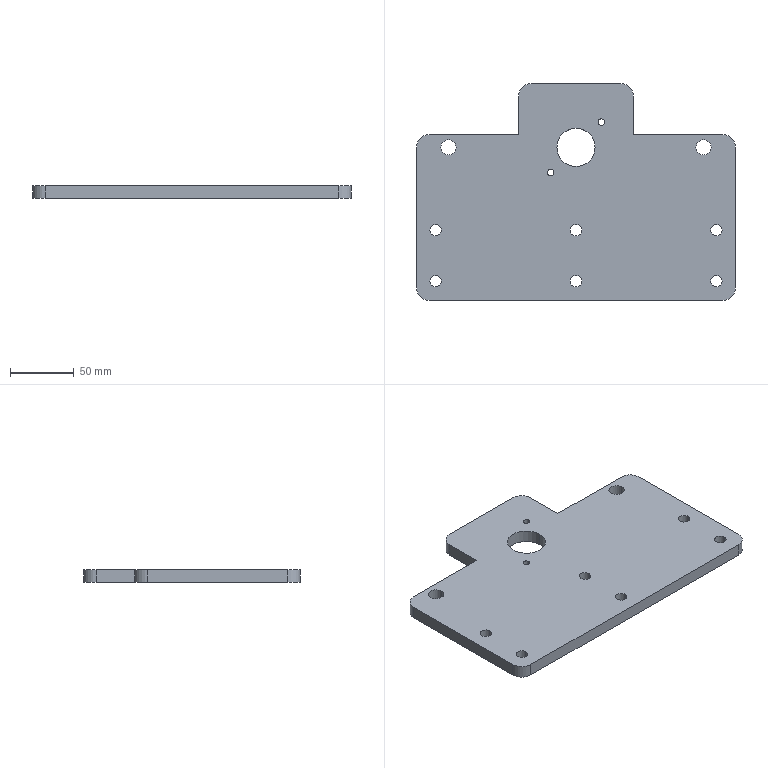Part | SolidWorks | features HoleWzd 3, ICE 2, Extrusion 1, Fillet 1, LPattern 1, MirrorPattern 1 | 1 solid | 38 faces | box 250 x 170 x 10 mm | volume 346172 mm3 | cylinder 28 | plane 10 | commonest cylinder face diameters 9 x12 20 x6 5 x4 12 x4 30 x2
STEP:
#1=CARTESIAN_POINT('',(-22.3,15.2,-5.));
#2=VERTEX_POINT('',#1);
#3=CARTESIAN_POINT('',(-17.3,15.2,-5.));
#4=VERTEX_POINT('',#3);
#5=CARTESIAN_POINT('',(-19.8,15.2,-5.));
#6=DIRECTION('',(0.,0.,1.));
#7=DIRECTION('',(1.,0.,0.));
#8=AXIS2_PLACEMENT_3D('',#5,#6,#7);
#9=CIRCLE('',#8,2.5);
#10=EDGE_CURVE('',#2,#4,#9,.T.);
#11=ORIENTED_EDGE('',*,*,#10,.F.);
#12=CARTESIAN_POINT('',(-22.3,15.2,5.));
#13=VERTEX_POINT('',#12);
#14=CARTESIAN_POINT('',(-22.3,15.2,5.));
#15=DIRECTION('',(0.,0.,1.));
#16=VECTOR('',#15,1000.);
#17=LINE('',#14,#16);
#18=EDGE_CURVE('',#2,#13,#17,.T.);
#19=ORIENTED_EDGE('',*,*,#18,.T.);
#20=CARTESIAN_POINT('',(-17.3,15.2,5.));
#21=VERTEX_POINT('',#20);
#22=CARTESIAN_POINT('',(-19.8,15.2,5.));
#23=DIRECTION('',(0.,0.,1.));
#24=DIRECTION('',(1.,0.,0.));
#25=AXIS2_PLACEMENT_3D('',#22,#23,#24);
#26=CIRCLE('',#25,2.5);
#27=EDGE_CURVE('',#13,#21,#26,.T.);
#28=ORIENTED_EDGE('',*,*,#27,.T.);
#29=CARTESIAN_POINT('',(-17.3,15.2,5.));
#30=DIRECTION('',(0.,0.,1.));
#31=VECTOR('',#30,1000.);
#32=LINE('',#29,#31);
#33=EDGE_CURVE('',#4,#21,#32,.T.);
#34=ORIENTED_EDGE('',*,*,#33,.F.);
#35=EDGE_LOOP('',(#11,#19,#28,#34));
#36=FACE_OUTER_BOUND('',#35,.T.);
#37=CARTESIAN_POINT('',(-19.8,15.2,5.));
#38=DIRECTION('',(0.,0.,1.));
#39=DIRECTION('',(1.,0.,0.));
#40=AXIS2_PLACEMENT_3D('',#37,#38,#39);
#41=CYLINDRICAL_SURFACE('',#40,2.5);
#42=ADVANCED_FACE('',(#36),#41,.F.);
#43=CARTESIAN_POINT('',(17.3,54.8,-5.));
#44=VERTEX_POINT('',#43);
#45=CARTESIAN_POINT('',(22.3,54.8,-5.));
#46=VERTEX_POINT('',#45);
#47=CARTESIAN_POINT('',(19.8,54.8,-5.));
#48=DIRECTION('',(0.,0.,1.));
#49=DIRECTION('',(1.,0.,0.));
#50=AXIS2_PLACEMENT_3D('',#47,#48,#49);
#51=CIRCLE('',#50,2.5);
#52=EDGE_CURVE('',#44,#46,#51,.T.);
#53=ORIENTED_EDGE('',*,*,#52,.F.);
#54=CARTESIAN_POINT('',(17.3,54.8,5.));
#55=VERTEX_POINT('',#54);
#56=CARTESIAN_POINT('',(17.3,54.8,5.));
#57=DIRECTION('',(0.,0.,1.));
#58=VECTOR('',#57,1000.);
#59=LINE('',#56,#58);
#60=EDGE_CURVE('',#44,#55,#59,.T.);
#61=ORIENTED_EDGE('',*,*,#60,.T.);
#62=CARTESIAN_POINT('',(22.3,54.8,5.));
#63=VERTEX_POINT('',#62);
#64=CARTESIAN_POINT('',(19.8,54.8,5.));
#65=DIRECTION('',(0.,0.,1.));
#66=DIRECTION('',(1.,0.,0.));
#67=AXIS2_PLACEMENT_3D('',#64,#65,#66);
#68=CIRCLE('',#67,2.5);
#69=EDGE_CURVE('',#55,#63,#68,.T.);
#70=ORIENTED_EDGE('',*,*,#69,.T.);
#71=CARTESIAN_POINT('',(22.3,54.8,5.));
#72=DIRECTION('',(0.,0.,1.));
#73=VECTOR('',#72,1000.);
#74=LINE('',#71,#73);
#75=EDGE_CURVE('',#46,#63,#74,.T.);
#76=ORIENTED_EDGE('',*,*,#75,.F.);
#77=EDGE_LOOP('',(#53,#61,#70,#76));
#78=FACE_OUTER_BOUND('',#77,.T.);
#79=CARTESIAN_POINT('',(19.8,54.8,5.));
#80=DIRECTION('',(0.,0.,1.));
#81=DIRECTION('',(1.,0.,0.));
#82=AXIS2_PLACEMENT_3D('',#79,#80,#81);
#83=CYLINDRICAL_SURFACE('',#82,2.5);
#84=ADVANCED_FACE('',(#78),#83,.F.);
#85=CARTESIAN_POINT('',(-15.,35.,-5.));
#86=VERTEX_POINT('',#85);
#87=CARTESIAN_POINT('',(15.,35.,-5.));
#88=VERTEX_POINT('',#87);
#89=CARTESIAN_POINT('',(0.,35.,-5.));
#90=DIRECTION('',(0.,0.,1.));
#91=DIRECTION('',(1.,0.,0.));
#92=AXIS2_PLACEMENT_3D('',#89,#90,#91);
#93=CIRCLE('',#92,15.);
#94=EDGE_CURVE('',#86,#88,#93,.T.);
#95=ORIENTED_EDGE('',*,*,#94,.F.);
#96=CARTESIAN_POINT('',(-15.,35.,5.));
#97=VERTEX_POINT('',#96);
#98=CARTESIAN_POINT('',(-15.,35.,-5.));
#99=DIRECTION('',(0.,0.,1.));
#100=VECTOR('',#99,1000.);
#101=LINE('',#98,#100);
#102=EDGE_CURVE('',#86,#97,#101,.T.);
#103=ORIENTED_EDGE('',*,*,#102,.T.);
#104=CARTESIAN_POINT('',(15.,35.,5.));
#105=VERTEX_POINT('',#104);
#106=CARTESIAN_POINT('',(0.,35.,5.));
#107=DIRECTION('',(0.,0.,1.));
#108=DIRECTION('',(1.,0.,0.));
#109=AXIS2_PLACEMENT_3D('',#106,#107,#108);
#110=CIRCLE('',#109,15.);
#111=EDGE_CURVE('',#97,#105,#110,.T.);
#112=ORIENTED_EDGE('',*,*,#111,.T.);
#113=CARTESIAN_POINT('',(15.,35.,-5.));
#114=DIRECTION('',(0.,0.,1.));
#115=VECTOR('',#114,1000.);
#116=LINE('',#113,#115);
#117=EDGE_CURVE('',#88,#105,#116,.T.);
#118=ORIENTED_EDGE('',*,*,#117,.F.);
#119=EDGE_LOOP('',(#95,#103,#112,#118));
#120=FACE_OUTER_BOUND('',#119,.T.);
#121=CARTESIAN_POINT('',(0.,35.,-5.));
#122=DIRECTION('',(0.,0.,1.));
#123=DIRECTION('',(1.,0.,0.));
#124=AXIS2_PLACEMENT_3D('',#121,#122,#123);
#125=CYLINDRICAL_SURFACE('',#124,15.);
#126=ADVANCED_FACE('',(#120),#125,.F.);
#127=CARTESIAN_POINT('',(-106.,35.,-5.));
#128=VERTEX_POINT('',#127);
#129=CARTESIAN_POINT('',(-94.,35.,-5.));
#130=VERTEX_POINT('',#129);
#131=CARTESIAN_POINT('',(-100.,35.,-5.));
#132=DIRECTION('',(0.,0.,1.));
#133=DIRECTION('',(1.,0.,0.));
#134=AXIS2_PLACEMENT_3D('',#131,#132,#133);
#135=CIRCLE('',#134,6.);
#136=EDGE_CURVE('',#128,#130,#135,.T.);
#137=ORIENTED_EDGE('',*,*,#136,.F.);
#138=CARTESIAN_POINT('',(-106.,35.,5.));
#139=VERTEX_POINT('',#138);
#140=CARTESIAN_POINT('',(-106.,35.,5.));
#141=DIRECTION('',(0.,0.,1.));
#142=VECTOR('',#141,1000.);
#143=LINE('',#140,#142);
#144=EDGE_CURVE('',#128,#139,#143,.T.);
#145=ORIENTED_EDGE('',*,*,#144,.T.);
#146=CARTESIAN_POINT('',(-94.,35.,5.));
#147=VERTEX_POINT('',#146);
#148=CARTESIAN_POINT('',(-100.,35.,5.));
#149=DIRECTION('',(0.,0.,1.));
#150=DIRECTION('',(1.,0.,0.));
#151=AXIS2_PLACEMENT_3D('',#148,#149,#150);
#152=CIRCLE('',#151,6.);
#153=EDGE_CURVE('',#139,#147,#152,.T.);
#154=ORIENTED_EDGE('',*,*,#153,.T.);
#155=CARTESIAN_POINT('',(-94.,35.,5.));
#156=DIRECTION('',(0.,0.,1.));
#157=VECTOR('',#156,1000.);
#158=LINE('',#155,#157);
#159=EDGE_CURVE('',#130,#147,#158,.T.);
#160=ORIENTED_EDGE('',*,*,#159,.F.);
#161=EDGE_LOOP('',(#137,#145,#154,#160));
#162=FACE_OUTER_BOUND('',#161,.T.);
#163=CARTESIAN_POINT('',(-100.,35.,5.));
#164=DIRECTION('',(0.,0.,1.));
#165=DIRECTION('',(1.,0.,0.));
#166=AXIS2_PLACEMENT_3D('',#163,#164,#165);
#167=CYLINDRICAL_SURFACE('',#166,6.);
#168=ADVANCED_FACE('',(#162),#167,.F.);
#169=CARTESIAN_POINT('',(94.,35.,-5.));
#170=VERTEX_POINT('',#169);
#171=CARTESIAN_POINT('',(106.,35.,-5.));
#172=VERTEX_POINT('',#171);
#173=CARTESIAN_POINT('',(100.,35.,-5.));
#174=DIRECTION('',(0.,0.,1.));
#175=DIRECTION('',(1.,0.,0.));
#176=AXIS2_PLACEMENT_3D('',#173,#174,#175);
#177=CIRCLE('',#176,6.);
#178=EDGE_CURVE('',#170,#172,#177,.T.);
#179=ORIENTED_EDGE('',*,*,#178,.F.);
#180=CARTESIAN_POINT('',(94.,35.,5.));
#181=VERTEX_POINT('',#180);
#182=CARTESIAN_POINT('',(94.,35.,5.));
#183=DIRECTION('',(0.,0.,1.));
#184=VECTOR('',#183,1000.);
#185=LINE('',#182,#184);
#186=EDGE_CURVE('',#170,#181,#185,.T.);
#187=ORIENTED_EDGE('',*,*,#186,.T.);
#188=CARTESIAN_POINT('',(106.,35.,5.));
#189=VERTEX_POINT('',#188);
#190=CARTESIAN_POINT('',(100.,35.,5.));
#191=DIRECTION('',(0.,0.,1.));
#192=DIRECTION('',(1.,0.,0.));
#193=AXIS2_PLACEMENT_3D('',#190,#191,#192);
#194=CIRCLE('',#193,6.);
#195=EDGE_CURVE('',#181,#189,#194,.T.);
#196=ORIENTED_EDGE('',*,*,#195,.T.);
#197=CARTESIAN_POINT('',(106.,35.,5.));
#198=DIRECTION('',(0.,0.,1.));
#199=VECTOR('',#198,1000.);
#200=LINE('',#197,#199);
#201=EDGE_CURVE('',#172,#189,#200,.T.);
#202=ORIENTED_EDGE('',*,*,#201,.F.);
#203=EDGE_LOOP('',(#179,#187,#196,#202));
#204=FACE_OUTER_BOUND('',#203,.T.);
#205=CARTESIAN_POINT('',(100.,35.,5.));
#206=DIRECTION('',(0.,0.,1.));
#207=DIRECTION('',(1.,0.,0.));
#208=AXIS2_PLACEMENT_3D('',#205,#206,#207);
#209=CYLINDRICAL_SURFACE('',#208,6.);
#210=ADVANCED_FACE('',(#204),#209,.F.);
#211=CARTESIAN_POINT('',(105.5,-70.,-5.));
#212=VERTEX_POINT('',#211);
#213=CARTESIAN_POINT('',(114.5,-70.,-5.));
#214=VERTEX_POINT('',#213);
#215=CARTESIAN_POINT('',(110.,-70.,-5.));
#216=DIRECTION('',(0.,0.,1.));
#217=DIRECTION('',(1.,0.,0.));
#218=AXIS2_PLACEMENT_3D('',#215,#216,#217);
#219=CIRCLE('',#218,4.5);
#220=EDGE_CURVE('',#212,#214,#219,.T.);
#221=ORIENTED_EDGE('',*,*,#220,.F.);
#222=CARTESIAN_POINT('',(105.5,-70.,5.));
#223=VERTEX_POINT('',#222);
#224=CARTESIAN_POINT('',(105.5,-70.,5.));
#225=DIRECTION('',(0.,0.,1.));
#226=VECTOR('',#225,1000.);
#227=LINE('',#224,#226);
#228=EDGE_CURVE('',#212,#223,#227,.T.);
#229=ORIENTED_EDGE('',*,*,#228,.T.);
#230=CARTESIAN_POINT('',(114.5,-70.,5.));
#231=VERTEX_POINT('',#230);
#232=CARTESIAN_POINT('',(110.,-70.,5.));
#233=DIRECTION('',(0.,0.,1.));
#234=DIRECTION('',(1.,0.,0.));
#235=AXIS2_PLACEMENT_3D('',#232,#233,#234);
#236=CIRCLE('',#235,4.5);
#237=EDGE_CURVE('',#223,#231,#236,.T.);
#238=ORIENTED_EDGE('',*,*,#237,.T.);
#239=CARTESIAN_POINT('',(114.5,-70.,5.));
#240=DIRECTION('',(0.,0.,1.));
#241=VECTOR('',#240,1000.);
#242=LINE('',#239,#241);
#243=EDGE_CURVE('',#214,#231,#242,.T.);
#244=ORIENTED_EDGE('',*,*,#243,.F.);
#245=EDGE_LOOP('',(#221,#229,#238,#244));
#246=FACE_OUTER_BOUND('',#245,.T.);
#247=CARTESIAN_POINT('',(110.,-70.,5.));
#248=DIRECTION('',(0.,0.,1.));
#249=DIRECTION('',(1.,0.,0.));
#250=AXIS2_PLACEMENT_3D('',#247,#248,#249);
#251=CYLINDRICAL_SURFACE('',#250,4.5);
#252=ADVANCED_FACE('',(#246),#251,.F.);
#253=CARTESIAN_POINT('',(-4.5,-70.,-5.));
#254=VERTEX_POINT('',#253);
#255=CARTESIAN_POINT('',(4.5,-70.,-5.));
#256=VERTEX_POINT('',#255);
#257=CARTESIAN_POINT('',(0.,-70.,-5.));
#258=DIRECTION('',(0.,0.,1.));
#259=DIRECTION('',(1.,0.,0.));
#260=AXIS2_PLACEMENT_3D('',#257,#258,#259);
#261=CIRCLE('',#260,4.5);
#262=EDGE_CURVE('',#254,#256,#261,.T.);
#263=ORIENTED_EDGE('',*,*,#262,.F.);
#264=CARTESIAN_POINT('',(-4.5,-70.,5.));
#265=VERTEX_POINT('',#264);
#266=CARTESIAN_POINT('',(-4.5,-70.,5.));
#267=DIRECTION('',(0.,0.,1.));
#268=VECTOR('',#267,1000.);
#269=LINE('',#266,#268);
#270=EDGE_CURVE('',#254,#265,#269,.T.);
#271=ORIENTED_EDGE('',*,*,#270,.T.);
#272=CARTESIAN_POINT('',(4.5,-70.,5.));
#273=VERTEX_POINT('',#272);
#274=CARTESIAN_POINT('',(0.,-70.,5.));
#275=DIRECTION('',(0.,0.,1.));
#276=DIRECTION('',(1.,0.,0.));
#277=AXIS2_PLACEMENT_3D('',#274,#275,#276);
#278=CIRCLE('',#277,4.5);
#279=EDGE_CURVE('',#265,#273,#278,.T.);
#280=ORIENTED_EDGE('',*,*,#279,.T.);
#281=CARTESIAN_POINT('',(4.5,-70.,5.));
#282=DIRECTION('',(0.,0.,1.));
#283=VECTOR('',#282,1000.);
#284=LINE('',#281,#283);
#285=EDGE_CURVE('',#256,#273,#284,.T.);
#286=ORIENTED_EDGE('',*,*,#285,.F.);
#287=EDGE_LOOP('',(#263,#271,#280,#286));
#288=FACE_OUTER_BOUND('',#287,.T.);
#289=CARTESIAN_POINT('',(0.,-70.,5.));
#290=DIRECTION('',(0.,0.,1.));
#291=DIRECTION('',(1.,0.,0.));
#292=AXIS2_PLACEMENT_3D('',#289,#290,#291);
#293=CYLINDRICAL_SURFACE('',#292,4.5);
#294=ADVANCED_FACE('',(#288),#293,.F.);
#295=CARTESIAN_POINT('',(105.5,-30.,-5.));
#296=VERTEX_POINT('',#295);
#297=CARTESIAN_POINT('',(114.5,-30.,-5.));
#298=VERTEX_POINT('',#297);
#299=CARTESIAN_POINT('',(110.,-30.,-5.));
#300=DIRECTION('',(0.,0.,1.));
#301=DIRECTION('',(1.,0.,0.));
#302=AXIS2_PLACEMENT_3D('',#299,#300,#301);
#303=CIRCLE('',#302,4.5);
#304=EDGE_CURVE('',#296,#298,#303,.T.);
#305=ORIENTED_EDGE('',*,*,#304,.F.);
#306=CARTESIAN_POINT('',(105.5,-30.,5.));
#307=VERTEX_POINT('',#306);
#308=CARTESIAN_POINT('',(105.5,-30.,5.));
#309=DIRECTION('',(0.,0.,1.));
#310=VECTOR('',#309,1000.);
#311=LINE('',#308,#310);
#312=EDGE_CURVE('',#296,#307,#311,.T.);
#313=ORIENTED_EDGE('',*,*,#312,.T.);
#314=CARTESIAN_POINT('',(114.5,-30.,5.));
#315=VERTEX_POINT('',#314);
#316=CARTESIAN_POINT('',(110.,-30.,5.));
#317=DIRECTION('',(0.,0.,1.));
#318=DIRECTION('',(1.,0.,0.));
#319=AXIS2_PLACEMENT_3D('',#316,#317,#318);
#320=CIRCLE('',#319,4.5);
#321=EDGE_CURVE('',#307,#315,#320,.T.);
#322=ORIENTED_EDGE('',*,*,#321,.T.);
#323=CARTESIAN_POINT('',(114.5,-30.,5.));
#324=DIRECTION('',(0.,0.,1.));
#325=VECTOR('',#324,1000.);
#326=LINE('',#323,#325);
#327=EDGE_CURVE('',#298,#315,#326,.T.);
#328=ORIENTED_EDGE('',*,*,#327,.F.);
#329=EDGE_LOOP('',(#305,#313,#322,#328));
#330=FACE_OUTER_BOUND('',#329,.T.);
#331=CARTESIAN_POINT('',(110.,-30.,5.));
#332=DIRECTION('',(0.,0.,1.));
#333=DIRECTION('',(1.,0.,0.));
#334=AXIS2_PLACEMENT_3D('',#331,#332,#333);
#335=CYLINDRICAL_SURFACE('',#334,4.5);
#336=ADVANCED_FACE('',(#330),#335,.F.);
#337=CARTESIAN_POINT('',(-4.5,-30.,-5.));
#338=VERTEX_POINT('',#337);
#339=CARTESIAN_POINT('',(4.5,-30.,-5.));
#340=VERTEX_POINT('',#339);
#341=CARTESIAN_POINT('',(0.,-30.,-5.));
#342=DIRECTION('',(0.,0.,1.));
#343=DIRECTION('',(1.,0.,0.));
#344=AXIS2_PLACEMENT_3D('',#341,#342,#343);
#345=CIRCLE('',#344,4.5);
#346=EDGE_CURVE('',#338,#340,#345,.T.);
#347=ORIENTED_EDGE('',*,*,#346,.F.);
#348=CARTESIAN_POINT('',(-4.5,-30.,5.));
#349=VERTEX_POINT('',#348);
#350=CARTESIAN_POINT('',(-4.5,-30.,5.));
#351=DIRECTION('',(0.,0.,1.));
#352=VECTOR('',#351,1000.);
#353=LINE('',#350,#352);
#354=EDGE_CURVE('',#338,#349,#353,.T.);
#355=ORIENTED_EDGE('',*,*,#354,.T.);
#356=CARTESIAN_POINT('',(4.5,-30.,5.));
#357=VERTEX_POINT('',#356);
#358=CARTESIAN_POINT('',(0.,-30.,5.));
#359=DIRECTION('',(0.,0.,1.));
#360=DIRECTION('',(1.,0.,0.));
#361=AXIS2_PLACEMENT_3D('',#358,#359,#360);
#362=CIRCLE('',#361,4.5);
#363=EDGE_CURVE('',#349,#357,#362,.T.);
#364=ORIENTED_EDGE('',*,*,#363,.T.);
#365=CARTESIAN_POINT('',(4.5,-30.,5.));
#366=DIRECTION('',(0.,0.,1.));
#367=VECTOR('',#366,1000.);
#368=LINE('',#365,#367);
#369=EDGE_CURVE('',#340,#357,#368,.T.);
#370=ORIENTED_EDGE('',*,*,#369,.F.);
#371=EDGE_LOOP('',(#347,#355,#364,#370));
#372=FACE_OUTER_BOUND('',#371,.T.);
#373=CARTESIAN_POINT('',(0.,-30.,5.));
#374=DIRECTION('',(0.,0.,1.));
#375=DIRECTION('',(1.,0.,0.));
#376=AXIS2_PLACEMENT_3D('',#373,#374,#375);
#377=CYLINDRICAL_SURFACE('',#376,4.5);
#378=ADVANCED_FACE('',(#372),#377,.F.);
#379=CARTESIAN_POINT('',(-114.5,-30.,-5.));
#380=VERTEX_POINT('',#379);
#381=CARTESIAN_POINT('',(-105.5,-30.,-5.));
#382=VERTEX_POINT('',#381);
#383=CARTESIAN_POINT('',(-110.,-30.,-5.));
#384=DIRECTION('',(0.,0.,1.));
#385=DIRECTION('',(1.,0.,0.));
#386=AXIS2_PLACEMENT_3D('',#383,#384,#385);
#387=CIRCLE('',#386,4.5);
#388=EDGE_CURVE('',#380,#382,#387,.T.);
#389=ORIENTED_EDGE('',*,*,#388,.F.);
#390=CARTESIAN_POINT('',(-114.5,-30.,5.));
#391=VERTEX_POINT('',#390);
#392=CARTESIAN_POINT('',(-114.5,-30.,5.));
#393=DIRECTION('',(0.,0.,1.));
#394=VECTOR('',#393,1000.);
#395=LINE('',#392,#394);
#396=EDGE_CURVE('',#380,#391,#395,.T.);
#397=ORIENTED_EDGE('',*,*,#396,.T.);
#398=CARTESIAN_POINT('',(-105.5,-30.,5.));
#399=VERTEX_POINT('',#398);
#400=CARTESIAN_POINT('',(-110.,-30.,5.));
#401=DIRECTION('',(0.,0.,1.));
#402=DIRECTION('',(1.,0.,0.));
#403=AXIS2_PLACEMENT_3D('',#400,#401,#402);
#404=CIRCLE('',#403,4.5);
#405=EDGE_CURVE('',#391,#399,#404,.T.);
#406=ORIENTED_EDGE('',*,*,#405,.T.);
#407=CARTESIAN_POINT('',(-105.5,-30.,5.));
#408=DIRECTION('',(0.,0.,1.));
#409=VECTOR('',#408,1000.);
#410=LINE('',#407,#409);
#411=EDGE_CURVE('',#382,#399,#410,.T.);
#412=ORIENTED_EDGE('',*,*,#411,.F.);
#413=EDGE_LOOP('',(#389,#397,#406,#412));
#414=FACE_OUTER_BOUND('',#413,.T.);
#415=CARTESIAN_POINT('',(-110.,-30.,5.));
#416=DIRECTION('',(0.,0.,1.));
#417=DIRECTION('',(1.,0.,0.));
#418=AXIS2_PLACEMENT_3D('',#415,#416,#417);
#419=CYLINDRICAL_SURFACE('',#418,4.5);
#420=ADVANCED_FACE('',(#414),#419,.F.);
#421=CARTESIAN_POINT('',(-114.5,-70.,-5.));
#422=VERTEX_POINT('',#421);
#423=CARTESIAN_POINT('',(-105.5,-70.,-5.));
#424=VERTEX_POINT('',#423);
#425=CARTESIAN_POINT('',(-110.,-70.,-5.));
#426=DIRECTION('',(0.,0.,1.));
#427=DIRECTION('',(1.,0.,0.));
#428=AXIS2_PLACEMENT_3D('',#425,#426,#427);
#429=CIRCLE('',#428,4.5);
#430=EDGE_CURVE('',#422,#424,#429,.T.);
#431=ORIENTED_EDGE('',*,*,#430,.F.);
#432=CARTESIAN_POINT('',(-114.5,-70.,5.));
#433=VERTEX_POINT('',#432);
#434=CARTESIAN_POINT('',(-114.5,-70.,5.));
#435=DIRECTION('',(0.,0.,1.));
#436=VECTOR('',#435,1000.);
#437=LINE('',#434,#436);
#438=EDGE_CURVE('',#422,#433,#437,.T.);
#439=ORIENTED_EDGE('',*,*,#438,.T.);
#440=CARTESIAN_POINT('',(-105.5,-70.,5.));
#441=VERTEX_POINT('',#440);
#442=CARTESIAN_POINT('',(-110.,-70.,5.));
#443=DIRECTION('',(0.,0.,1.));
#444=DIRECTION('',(1.,0.,0.));
#445=AXIS2_PLACEMENT_3D('',#442,#443,#444);
#446=CIRCLE('',#445,4.5);
#447=EDGE_CURVE('',#433,#441,#446,.T.);
#448=ORIENTED_EDGE('',*,*,#447,.T.);
#449=CARTESIAN_POINT('',(-105.5,-70.,5.));
#450=DIRECTION('',(0.,0.,1.));
#451=VECTOR('',#450,1000.);
#452=LINE('',#449,#451);
#453=EDGE_CURVE('',#424,#441,#452,.T.);
#454=ORIENTED_EDGE('',*,*,#453,.F.);
#455=EDGE_LOOP('',(#431,#439,#448,#454));
#456=FACE_OUTER_BOUND('',#455,.T.);
#457=CARTESIAN_POINT('',(-110.,-70.,5.));
#458=DIRECTION('',(0.,0.,1.));
#459=DIRECTION('',(1.,0.,0.));
#460=AXIS2_PLACEMENT_3D('',#457,#458,#459);
#461=CYLINDRICAL_SURFACE('',#460,4.5);
#462=ADVANCED_FACE('',(#456),#461,.F.);
#463=CARTESIAN_POINT('',(35.,85.,5.));
#464=VERTEX_POINT('',#463);
#465=CARTESIAN_POINT('',(-35.,85.,5.));
#466=VERTEX_POINT('',#465);
#467=CARTESIAN_POINT('',(-125.,85.,5.));
#468=DIRECTION('',(-1.,0.,0.));
#469=VECTOR('',#468,1000.);
#470=LINE('',#467,#469);
#471=EDGE_CURVE('',#464,#466,#470,.T.);
#472=ORIENTED_EDGE('',*,*,#471,.F.);
#473=CARTESIAN_POINT('',(35.,85.,-5.));
#474=VERTEX_POINT('',#473);
#475=CARTESIAN_POINT('',(35.,85.,5.));
#476=DIRECTION('',(0.,0.,-1.));
#477=VECTOR('',#476,1000.);
#478=LINE('',#475,#477);
#479=EDGE_CURVE('',#464,#474,#478,.T.);
#480=ORIENTED_EDGE('',*,*,#479,.T.);
#481=CARTESIAN_POINT('',(-35.,85.,-5.));
#482=VERTEX_POINT('',#481);
#483=CARTESIAN_POINT('',(-125.,85.,-5.));
#484=DIRECTION('',(-1.,0.,0.));
#485=VECTOR('',#484,1000.);
#486=LINE('',#483,#485);
#487=EDGE_CURVE('',#474,#482,#486,.T.);
#488=ORIENTED_EDGE('',*,*,#487,.T.);
#489=CARTESIAN_POINT('',(-35.,85.,5.));
#490=DIRECTION('',(0.,0.,1.));
#491=VECTOR('',#490,1000.);
#492=LINE('',#489,#491);
#493=EDGE_CURVE('',#482,#466,#492,.T.);
#494=ORIENTED_EDGE('',*,*,#493,.T.);
#495=EDGE_LOOP('',(#472,#480,#488,#494));
#496=FACE_OUTER_BOUND('',#495,.T.);
#497=CARTESIAN_POINT('',(-125.,85.,5.));
#498=DIRECTION('',(0.,-1.,0.));
#499=DIRECTION('',(0.,0.,-1.));
#500=AXIS2_PLACEMENT_3D('',#497,#498,#499);
#501=PLANE('',#500);
#502=ADVANCED_FACE('',(#496),#501,.F.);
#503=CARTESIAN_POINT('',(-125.,35.,-5.));
#504=VERTEX_POINT('',#503);
#505=CARTESIAN_POINT('',(-125.,-75.,-5.));
#506=VERTEX_POINT('',#505);
#507=CARTESIAN_POINT('',(-125.,85.,-5.));
#508=DIRECTION('',(0.,-1.,0.));
#509=VECTOR('',#508,1000.);
#510=LINE('',#507,#509);
#511=EDGE_CURVE('',#504,#506,#510,.T.);
#512=ORIENTED_EDGE('',*,*,#511,.T.);
#513=CARTESIAN_POINT('',(-125.,-75.,5.));
#514=VERTEX_POINT('',#513);
#515=CARTESIAN_POINT('',(-125.,-75.,5.));
#516=DIRECTION('',(0.,0.,1.));
#517=VECTOR('',#516,1000.);
#518=LINE('',#515,#517);
#519=EDGE_CURVE('',#506,#514,#518,.T.);
#520=ORIENTED_EDGE('',*,*,#519,.T.);
#521=CARTESIAN_POINT('',(-125.,35.,5.));
#522=VERTEX_POINT('',#521);
#523=CARTESIAN_POINT('',(-125.,85.,5.));
#524=DIRECTION('',(0.,-1.,0.));
#525=VECTOR('',#524,1000.);
#526=LINE('',#523,#525);
#527=EDGE_CURVE('',#522,#514,#526,.T.);
#528=ORIENTED_EDGE('',*,*,#527,.F.);
#529=CARTESIAN_POINT('',(-125.,35.,-5.));
#530=DIRECTION('',(0.,0.,-1.));
#531=VECTOR('',#530,1000.);
#532=LINE('',#529,#531);
#533=EDGE_CURVE('',#522,#504,#532,.T.);
#534=ORIENTED_EDGE('',*,*,#533,.T.);
#535=EDGE_LOOP('',(#512,#520,#528,#534));
#536=FACE_OUTER_BOUND('',#535,.T.);
#537=CARTESIAN_POINT('',(-125.,85.,5.));
#538=DIRECTION('',(1.,0.,0.));
#539=DIRECTION('',(0.,1.,0.));
#540=AXIS2_PLACEMENT_3D('',#537,#538,#539);
#541=PLANE('',#540);
#542=ADVANCED_FACE('',(#536),#541,.F.);
#543=CARTESIAN_POINT('',(-19.8,15.2,5.));
#544=DIRECTION('',(0.,0.,1.));
#545=DIRECTION('',(1.,0.,0.));
#546=AXIS2_PLACEMENT_3D('',#543,#544,#545);
#547=CIRCLE('',#546,2.5);
#548=EDGE_CURVE('',#21,#13,#547,.T.);
#549=ORIENTED_EDGE('',*,*,#548,.F.);
#550=ORIENTED_EDGE('',*,*,#27,.F.);
#551=EDGE_LOOP('',(#549,#550));
#552=FACE_BOUND('',#551,.T.);
#553=CARTESIAN_POINT('',(19.8,54.8,5.));
#554=DIRECTION('',(0.,0.,1.));
#555=DIRECTION('',(1.,0.,0.));
#556=AXIS2_PLACEMENT_3D('',#553,#554,#555);
#557=CIRCLE('',#556,2.5);
#558=EDGE_CURVE('',#63,#55,#557,.T.);
#559=ORIENTED_EDGE('',*,*,#558,.F.);
#560=ORIENTED_EDGE('',*,*,#69,.F.);
#561=EDGE_LOOP('',(#559,#560));
#562=FACE_BOUND('',#561,.T.);
#563=CARTESIAN_POINT('',(0.,35.,5.));
#564=DIRECTION('',(0.,0.,1.));
#565=DIRECTION('',(1.,0.,0.));
#566=AXIS2_PLACEMENT_3D('',#563,#564,#565);
#567=CIRCLE('',#566,15.);
#568=EDGE_CURVE('',#105,#97,#567,.T.);
#569=ORIENTED_EDGE('',*,*,#568,.F.);
#570=ORIENTED_EDGE('',*,*,#111,.F.);
#571=EDGE_LOOP('',(#569,#570));
#572=FACE_BOUND('',#571,.T.);
#573=CARTESIAN_POINT('',(-100.,35.,5.));
#574=DIRECTION('',(0.,0.,1.));
#575=DIRECTION('',(1.,0.,0.));
#576=AXIS2_PLACEMENT_3D('',#573,#574,#575);
#577=CIRCLE('',#576,6.);
#578=EDGE_CURVE('',#147,#139,#577,.T.);
#579=ORIENTED_EDGE('',*,*,#578,.F.);
#580=ORIENTED_EDGE('',*,*,#153,.F.);
#581=EDGE_LOOP('',(#579,#580));
#582=FACE_BOUND('',#581,.T.);
#583=CARTESIAN_POINT('',(100.,35.,5.));
#584=DIRECTION('',(0.,0.,1.));
#585=DIRECTION('',(1.,0.,0.));
#586=AXIS2_PLACEMENT_3D('',#583,#584,#585);
#587=CIRCLE('',#586,6.);
#588=EDGE_CURVE('',#189,#181,#587,.T.);
#589=ORIENTED_EDGE('',*,*,#588,.F.);
#590=ORIENTED_EDGE('',*,*,#195,.F.);
#591=EDGE_LOOP('',(#589,#590));
#592=FACE_BOUND('',#591,.T.);
#593=CARTESIAN_POINT('',(0.,-70.,5.));
#594=DIRECTION('',(0.,0.,1.));
#595=DIRECTION('',(1.,0.,0.));
#596=AXIS2_PLACEMENT_3D('',#593,#594,#595);
#597=CIRCLE('',#596,4.5);
#598=EDGE_CURVE('',#273,#265,#597,.T.);
#599=ORIENTED_EDGE('',*,*,#598,.F.);
#600=ORIENTED_EDGE('',*,*,#279,.F.);
#601=EDGE_LOOP('',(#599,#600));
#602=FACE_BOUND('',#601,.T.);
#603=CARTESIAN_POINT('',(0.,-30.,5.));
#604=DIRECTION('',(0.,0.,1.));
#605=DIRECTION('',(1.,0.,0.));
#606=AXIS2_PLACEMENT_3D('',#603,#604,#605);
#607=CIRCLE('',#606,4.5);
#608=EDGE_CURVE('',#357,#349,#607,.T.);
#609=ORIENTED_EDGE('',*,*,#608,.F.);
#610=ORIENTED_EDGE('',*,*,#363,.F.);
#611=EDGE_LOOP('',(#609,#610));
#612=FACE_BOUND('',#611,.T.);
#613=CARTESIAN_POINT('',(-110.,-30.,5.));
#614=DIRECTION('',(0.,0.,1.));
#615=DIRECTION('',(1.,0.,0.));
#616=AXIS2_PLACEMENT_3D('',#613,#614,#615);
#617=CIRCLE('',#616,4.5);
#618=EDGE_CURVE('',#399,#391,#617,.T.);
#619=ORIENTED_EDGE('',*,*,#618,.F.);
#620=ORIENTED_EDGE('',*,*,#405,.F.);
#621=EDGE_LOOP('',(#619,#620));
#622=FACE_BOUND('',#621,.T.);
#623=CARTESIAN_POINT('',(-110.,-70.,5.));
#624=DIRECTION('',(0.,0.,1.));
#625=DIRECTION('',(1.,0.,0.));
#626=AXIS2_PLACEMENT_3D('',#623,#624,#625);
#627=CIRCLE('',#626,4.5);
#628=EDGE_CURVE('',#441,#433,#627,.T.);
#629=ORIENTED_EDGE('',*,*,#628,.F.);
#630=ORIENTED_EDGE('',*,*,#447,.F.);
#631=EDGE_LOOP('',(#629,#630));
#632=FACE_BOUND('',#631,.T.);
#633=CARTESIAN_POINT('',(-115.,-85.,5.));
#634=VERTEX_POINT('',#633);
#635=CARTESIAN_POINT('',(115.,-85.,5.));
#636=VERTEX_POINT('',#635);
#637=CARTESIAN_POINT('',(-125.,-85.,5.));
#638=DIRECTION('',(1.,0.,0.));
#639=VECTOR('',#638,1000.);
#640=LINE('',#637,#639);
#641=EDGE_CURVE('',#634,#636,#640,.T.);
#642=ORIENTED_EDGE('',*,*,#641,.T.);
#643=CARTESIAN_POINT('',(125.,-75.,5.));
#644=VERTEX_POINT('',#643);
#645=CARTESIAN_POINT('',(115.,-75.,5.));
#646=DIRECTION('',(0.,0.,1.));
#647=DIRECTION('',(1.,0.,0.));
#648=AXIS2_PLACEMENT_3D('',#645,#646,#647);
#649=CIRCLE('',#648,10.);
#650=EDGE_CURVE('',#636,#644,#649,.T.);
#651=ORIENTED_EDGE('',*,*,#650,.T.);
#652=CARTESIAN_POINT('',(125.,35.,5.));
#653=VERTEX_POINT('',#652);
#654=CARTESIAN_POINT('',(125.,85.,5.));
#655=DIRECTION('',(0.,1.,0.));
#656=VECTOR('',#655,1000.);
#657=LINE('',#654,#656);
#658=EDGE_CURVE('',#644,#653,#657,.T.);
#659=ORIENTED_EDGE('',*,*,#658,.T.);
#660=CARTESIAN_POINT('',(115.,45.,5.));
#661=VERTEX_POINT('',#660);
#662=CARTESIAN_POINT('',(115.,35.,5.));
#663=DIRECTION('',(0.,0.,1.));
#664=DIRECTION('',(1.,0.,0.));
#665=AXIS2_PLACEMENT_3D('',#662,#663,#664);
#666=CIRCLE('',#665,10.);
#667=EDGE_CURVE('',#653,#661,#666,.T.);
#668=ORIENTED_EDGE('',*,*,#667,.T.);
#669=CARTESIAN_POINT('',(45.,45.,5.));
#670=VERTEX_POINT('',#669);
#671=CARTESIAN_POINT('',(45.,45.,5.));
#672=DIRECTION('',(1.,0.,0.));
#673=VECTOR('',#672,1000.);
#674=LINE('',#671,#673);
#675=EDGE_CURVE('',#670,#661,#674,.T.);
#676=ORIENTED_EDGE('',*,*,#675,.F.);
#677=CARTESIAN_POINT('',(45.,75.,5.));
#678=VERTEX_POINT('',#677);
#679=CARTESIAN_POINT('',(45.,85.,5.));
#680=DIRECTION('',(0.,-1.,0.));
#681=VECTOR('',#680,1000.);
#682=LINE('',#679,#681);
#683=EDGE_CURVE('',#678,#670,#682,.T.);
#684=ORIENTED_EDGE('',*,*,#683,.F.);
#685=CARTESIAN_POINT('',(35.,75.,5.));
#686=DIRECTION('',(0.,0.,1.));
#687=DIRECTION('',(1.,0.,0.));
#688=AXIS2_PLACEMENT_3D('',#685,#686,#687);
#689=CIRCLE('',#688,10.);
#690=EDGE_CURVE('',#678,#464,#689,.T.);
#691=ORIENTED_EDGE('',*,*,#690,.T.);
#692=ORIENTED_EDGE('',*,*,#471,.T.);
#693=CARTESIAN_POINT('',(-45.,75.,5.));
#694=VERTEX_POINT('',#693);
#695=CARTESIAN_POINT('',(-35.,75.,5.));
#696=DIRECTION('',(0.,0.,1.));
#697=DIRECTION('',(1.,0.,0.));
#698=AXIS2_PLACEMENT_3D('',#695,#696,#697);
#699=CIRCLE('',#698,10.);
#700=EDGE_CURVE('',#466,#694,#699,.T.);
#701=ORIENTED_EDGE('',*,*,#700,.T.);
#702=CARTESIAN_POINT('',(-45.,45.,5.));
#703=VERTEX_POINT('',#702);
#704=CARTESIAN_POINT('',(-45.,85.,5.));
#705=DIRECTION('',(0.,-1.,0.));
#706=VECTOR('',#705,1000.);
#707=LINE('',#704,#706);
#708=EDGE_CURVE('',#694,#703,#707,.T.);
#709=ORIENTED_EDGE('',*,*,#708,.T.);
#710=CARTESIAN_POINT('',(-115.,45.,5.));
#711=VERTEX_POINT('',#710);
#712=CARTESIAN_POINT('',(-45.,45.,5.));
#713=DIRECTION('',(-1.,0.,0.));
#714=VECTOR('',#713,1000.);
#715=LINE('',#712,#714);
#716=EDGE_CURVE('',#703,#711,#715,.T.);
#717=ORIENTED_EDGE('',*,*,#716,.T.);
#718=CARTESIAN_POINT('',(-115.,35.,5.));
#719=DIRECTION('',(0.,0.,1.));
#720=DIRECTION('',(1.,0.,0.));
#721=AXIS2_PLACEMENT_3D('',#718,#719,#720);
#722=CIRCLE('',#721,10.);
#723=EDGE_CURVE('',#711,#522,#722,.T.);
#724=ORIENTED_EDGE('',*,*,#723,.T.);
#725=ORIENTED_EDGE('',*,*,#527,.T.);
#726=CARTESIAN_POINT('',(-115.,-75.,5.));
#727=DIRECTION('',(0.,0.,1.));
#728=DIRECTION('',(1.,0.,0.));
#729=AXIS2_PLACEMENT_3D('',#726,#727,#728);
#730=CIRCLE('',#729,10.);
#731=EDGE_CURVE('',#514,#634,#730,.T.);
#732=ORIENTED_EDGE('',*,*,#731,.T.);
#733=EDGE_LOOP('',(#642,#651,#659,#668,#676,#684,#691,#692,#701,#709,#717,#724,#725,#732));
#734=FACE_OUTER_BOUND('',#733,.T.);
#735=CARTESIAN_POINT('',(110.,-30.,5.));
#736=DIRECTION('',(0.,0.,1.));
#737=DIRECTION('',(1.,0.,0.));
#738=AXIS2_PLACEMENT_3D('',#735,#736,#737);
#739=CIRCLE('',#738,4.5);
#740=EDGE_CURVE('',#315,#307,#739,.T.);
#741=ORIENTED_EDGE('',*,*,#740,.F.);
#742=ORIENTED_EDGE('',*,*,#321,.F.);
#743=EDGE_LOOP('',(#741,#742));
#744=FACE_BOUND('',#743,.T.);
#745=CARTESIAN_POINT('',(110.,-70.,5.));
#746=DIRECTION('',(0.,0.,1.));
#747=DIRECTION('',(1.,0.,0.));
#748=AXIS2_PLACEMENT_3D('',#745,#746,#747);
#749=CIRCLE('',#748,4.5);
#750=EDGE_CURVE('',#231,#223,#749,.T.);
#751=ORIENTED_EDGE('',*,*,#750,.F.);
#752=ORIENTED_EDGE('',*,*,#237,.F.);
#753=EDGE_LOOP('',(#751,#752));
#754=FACE_BOUND('',#753,.T.);
#755=CARTESIAN_POINT('',(0.,0.,5.));
#756=DIRECTION('',(0.,0.,1.));
#757=DIRECTION('',(1.,0.,0.));
#758=AXIS2_PLACEMENT_3D('',#755,#756,#757);
#759=PLANE('',#758);
#760=ADVANCED_FACE('',(#552,#562,#572,#582,#592,#602,#612,#622,#632,#734,#744,#754),#759,.T.);
#761=CARTESIAN_POINT('',(-19.8,15.2,-5.));
#762=DIRECTION('',(0.,0.,1.));
#763=DIRECTION('',(1.,0.,0.));
#764=AXIS2_PLACEMENT_3D('',#761,#762,#763);
#765=CIRCLE('',#764,2.5);
#766=EDGE_CURVE('',#4,#2,#765,.T.);
#767=ORIENTED_EDGE('',*,*,#766,.T.);
#768=ORIENTED_EDGE('',*,*,#10,.T.);
#769=EDGE_LOOP('',(#767,#768));
#770=FACE_BOUND('',#769,.T.);
#771=CARTESIAN_POINT('',(19.8,54.8,-5.));
#772=DIRECTION('',(0.,0.,1.));
#773=DIRECTION('',(1.,0.,0.));
#774=AXIS2_PLACEMENT_3D('',#771,#772,#773);
#775=CIRCLE('',#774,2.5);
#776=EDGE_CURVE('',#46,#44,#775,.T.);
#777=ORIENTED_EDGE('',*,*,#776,.T.);
#778=ORIENTED_EDGE('',*,*,#52,.T.);
#779=EDGE_LOOP('',(#777,#778));
#780=FACE_BOUND('',#779,.T.);
#781=CARTESIAN_POINT('',(0.,35.,-5.));
#782=DIRECTION('',(0.,0.,1.));
#783=DIRECTION('',(1.,0.,0.));
#784=AXIS2_PLACEMENT_3D('',#781,#782,#783);
#785=CIRCLE('',#784,15.);
#786=EDGE_CURVE('',#88,#86,#785,.T.);
#787=ORIENTED_EDGE('',*,*,#786,.T.);
#788=ORIENTED_EDGE('',*,*,#94,.T.);
#789=EDGE_LOOP('',(#787,#788));
#790=FACE_BOUND('',#789,.T.);
#791=CARTESIAN_POINT('',(-100.,35.,-5.));
#792=DIRECTION('',(0.,0.,1.));
#793=DIRECTION('',(1.,0.,0.));
#794=AXIS2_PLACEMENT_3D('',#791,#792,#793);
#795=CIRCLE('',#794,6.);
#796=EDGE_CURVE('',#130,#128,#795,.T.);
#797=ORIENTED_EDGE('',*,*,#796,.T.);
#798=ORIENTED_EDGE('',*,*,#136,.T.);
#799=EDGE_LOOP('',(#797,#798));
#800=FACE_BOUND('',#799,.T.);
#801=CARTESIAN_POINT('',(100.,35.,-5.));
#802=DIRECTION('',(0.,0.,1.));
#803=DIRECTION('',(1.,0.,0.));
#804=AXIS2_PLACEMENT_3D('',#801,#802,#803);
#805=CIRCLE('',#804,6.);
#806=EDGE_CURVE('',#172,#170,#805,.T.);
#807=ORIENTED_EDGE('',*,*,#806,.T.);
#808=ORIENTED_EDGE('',*,*,#178,.T.);
#809=EDGE_LOOP('',(#807,#808));
#810=FACE_BOUND('',#809,.T.);
#811=CARTESIAN_POINT('',(0.,-70.,-5.));
#812=DIRECTION('',(0.,0.,1.));
#813=DIRECTION('',(1.,0.,0.));
#814=AXIS2_PLACEMENT_3D('',#811,#812,#813);
#815=CIRCLE('',#814,4.5);
#816=EDGE_CURVE('',#256,#254,#815,.T.);
#817=ORIENTED_EDGE('',*,*,#816,.T.);
#818=ORIENTED_EDGE('',*,*,#262,.T.);
#819=EDGE_LOOP('',(#817,#818));
#820=FACE_BOUND('',#819,.T.);
#821=CARTESIAN_POINT('',(0.,-30.,-5.));
#822=DIRECTION('',(0.,0.,1.));
#823=DIRECTION('',(1.,0.,0.));
#824=AXIS2_PLACEMENT_3D('',#821,#822,#823);
#825=CIRCLE('',#824,4.5);
#826=EDGE_CURVE('',#340,#338,#825,.T.);
#827=ORIENTED_EDGE('',*,*,#826,.T.);
#828=ORIENTED_EDGE('',*,*,#346,.T.);
#829=EDGE_LOOP('',(#827,#828));
#830=FACE_BOUND('',#829,.T.);
#831=CARTESIAN_POINT('',(-110.,-30.,-5.));
#832=DIRECTION('',(0.,0.,1.));
#833=DIRECTION('',(1.,0.,0.));
#834=AXIS2_PLACEMENT_3D('',#831,#832,#833);
#835=CIRCLE('',#834,4.5);
#836=EDGE_CURVE('',#382,#380,#835,.T.);
#837=ORIENTED_EDGE('',*,*,#836,.T.);
#838=ORIENTED_EDGE('',*,*,#388,.T.);
#839=EDGE_LOOP('',(#837,#838));
#840=FACE_BOUND('',#839,.T.);
#841=CARTESIAN_POINT('',(-110.,-70.,-5.));
#842=DIRECTION('',(0.,0.,1.));
#843=DIRECTION('',(1.,0.,0.));
#844=AXIS2_PLACEMENT_3D('',#841,#842,#843);
#845=CIRCLE('',#844,4.5);
#846=EDGE_CURVE('',#424,#422,#845,.T.);
#847=ORIENTED_EDGE('',*,*,#846,.T.);
#848=ORIENTED_EDGE('',*,*,#430,.T.);
#849=EDGE_LOOP('',(#847,#848));
#850=FACE_BOUND('',#849,.T.);
#851=CARTESIAN_POINT('',(125.,-75.,-5.));
#852=VERTEX_POINT('',#851);
#853=CARTESIAN_POINT('',(125.,35.,-5.));
#854=VERTEX_POINT('',#853);
#855=CARTESIAN_POINT('',(125.,85.,-5.));
#856=DIRECTION('',(0.,1.,0.));
#857=VECTOR('',#856,1000.);
#858=LINE('',#855,#857);
#859=EDGE_CURVE('',#852,#854,#858,.T.);
#860=ORIENTED_EDGE('',*,*,#859,.F.);
#861=CARTESIAN_POINT('',(115.,-85.,-5.));
#862=VERTEX_POINT('',#861);
#863=CARTESIAN_POINT('',(115.,-75.,-5.));
#864=DIRECTION('',(0.,0.,-1.));
#865=DIRECTION('',(1.,0.,0.));
#866=AXIS2_PLACEMENT_3D('',#863,#864,#865);
#867=CIRCLE('',#866,10.);
#868=EDGE_CURVE('',#852,#862,#867,.T.);
#869=ORIENTED_EDGE('',*,*,#868,.T.);
#870=CARTESIAN_POINT('',(-115.,-85.,-5.));
#871=VERTEX_POINT('',#870);
#872=CARTESIAN_POINT('',(-125.,-85.,-5.));
#873=DIRECTION('',(1.,0.,0.));
#874=VECTOR('',#873,1000.);
#875=LINE('',#872,#874);
#876=EDGE_CURVE('',#871,#862,#875,.T.);
#877=ORIENTED_EDGE('',*,*,#876,.F.);
#878=CARTESIAN_POINT('',(-115.,-75.,-5.));
#879=DIRECTION('',(0.,0.,-1.));
#880=DIRECTION('',(1.,0.,0.));
#881=AXIS2_PLACEMENT_3D('',#878,#879,#880);
#882=CIRCLE('',#881,10.);
#883=EDGE_CURVE('',#871,#506,#882,.T.);
#884=ORIENTED_EDGE('',*,*,#883,.T.);
#885=ORIENTED_EDGE('',*,*,#511,.F.);
#886=CARTESIAN_POINT('',(-115.,45.,-5.));
#887=VERTEX_POINT('',#886);
#888=CARTESIAN_POINT('',(-115.,35.,-5.));
#889=DIRECTION('',(0.,0.,-1.));
#890=DIRECTION('',(1.,0.,0.));
#891=AXIS2_PLACEMENT_3D('',#888,#889,#890);
#892=CIRCLE('',#891,10.);
#893=EDGE_CURVE('',#504,#887,#892,.T.);
#894=ORIENTED_EDGE('',*,*,#893,.T.);
#895=CARTESIAN_POINT('',(-45.,45.,-5.));
#896=VERTEX_POINT('',#895);
#897=CARTESIAN_POINT('',(-45.,45.,-5.));
#898=DIRECTION('',(-1.,0.,0.));
#899=VECTOR('',#898,1000.);
#900=LINE('',#897,#899);
#901=EDGE_CURVE('',#896,#887,#900,.T.);
#902=ORIENTED_EDGE('',*,*,#901,.F.);
#903=CARTESIAN_POINT('',(-45.,75.,-5.));
#904=VERTEX_POINT('',#903);
#905=CARTESIAN_POINT('',(-45.,85.,-5.));
#906=DIRECTION('',(0.,-1.,0.));
#907=VECTOR('',#906,1000.);
#908=LINE('',#905,#907);
#909=EDGE_CURVE('',#904,#896,#908,.T.);
#910=ORIENTED_EDGE('',*,*,#909,.F.);
#911=CARTESIAN_POINT('',(-35.,75.,-5.));
#912=DIRECTION('',(0.,0.,-1.));
#913=DIRECTION('',(1.,0.,0.));
#914=AXIS2_PLACEMENT_3D('',#911,#912,#913);
#915=CIRCLE('',#914,10.);
#916=EDGE_CURVE('',#904,#482,#915,.T.);
#917=ORIENTED_EDGE('',*,*,#916,.T.);
#918=ORIENTED_EDGE('',*,*,#487,.F.);
#919=CARTESIAN_POINT('',(45.,75.,-5.));
#920=VERTEX_POINT('',#919);
#921=CARTESIAN_POINT('',(35.,75.,-5.));
#922=DIRECTION('',(0.,0.,-1.));
#923=DIRECTION('',(1.,0.,0.));
#924=AXIS2_PLACEMENT_3D('',#921,#922,#923);
#925=CIRCLE('',#924,10.);
#926=EDGE_CURVE('',#474,#920,#925,.T.);
#927=ORIENTED_EDGE('',*,*,#926,.T.);
#928=CARTESIAN_POINT('',(45.,45.,-5.));
#929=VERTEX_POINT('',#928);
#930=CARTESIAN_POINT('',(45.,85.,-5.));
#931=DIRECTION('',(0.,-1.,0.));
#932=VECTOR('',#931,1000.);
#933=LINE('',#930,#932);
#934=EDGE_CURVE('',#920,#929,#933,.T.);
#935=ORIENTED_EDGE('',*,*,#934,.T.);
#936=CARTESIAN_POINT('',(115.,45.,-5.));
#937=VERTEX_POINT('',#936);
#938=CARTESIAN_POINT('',(45.,45.,-5.));
#939=DIRECTION('',(1.,0.,0.));
#940=VECTOR('',#939,1000.);
#941=LINE('',#938,#940);
#942=EDGE_CURVE('',#929,#937,#941,.T.);
#943=ORIENTED_EDGE('',*,*,#942,.T.);
#944=CARTESIAN_POINT('',(115.,35.,-5.));
#945=DIRECTION('',(0.,0.,-1.));
#946=DIRECTION('',(1.,0.,0.));
#947=AXIS2_PLACEMENT_3D('',#944,#945,#946);
#948=CIRCLE('',#947,10.);
#949=EDGE_CURVE('',#937,#854,#948,.T.);
#950=ORIENTED_EDGE('',*,*,#949,.T.);
#951=EDGE_LOOP('',(#860,#869,#877,#884,#885,#894,#902,#910,#917,#918,#927,#935,#943,#950));
#952=FACE_OUTER_BOUND('',#951,.T.);
#953=CARTESIAN_POINT('',(110.,-30.,-5.));
#954=DIRECTION('',(0.,0.,1.));
#955=DIRECTION('',(1.,0.,0.));
#956=AXIS2_PLACEMENT_3D('',#953,#954,#955);
#957=CIRCLE('',#956,4.5);
#958=EDGE_CURVE('',#298,#296,#957,.T.);
#959=ORIENTED_EDGE('',*,*,#958,.T.);
#960=ORIENTED_EDGE('',*,*,#304,.T.);
#961=EDGE_LOOP('',(#959,#960));
#962=FACE_BOUND('',#961,.T.);
#963=CARTESIAN_POINT('',(110.,-70.,-5.));
#964=DIRECTION('',(0.,0.,1.));
#965=DIRECTION('',(1.,0.,0.));
#966=AXIS2_PLACEMENT_3D('',#963,#964,#965);
#967=CIRCLE('',#966,4.5);
#968=EDGE_CURVE('',#214,#212,#967,.T.);
#969=ORIENTED_EDGE('',*,*,#968,.T.);
#970=ORIENTED_EDGE('',*,*,#220,.T.);
#971=EDGE_LOOP('',(#969,#970));
#972=FACE_BOUND('',#971,.T.);
#973=CARTESIAN_POINT('',(0.,0.,-5.));
#974=DIRECTION('',(0.,0.,1.));
#975=DIRECTION('',(1.,0.,0.));
#976=AXIS2_PLACEMENT_3D('',#973,#974,#975);
#977=PLANE('',#976);
#978=ADVANCED_FACE('',(#770,#780,#790,#800,#810,#820,#830,#840,#850,#952,#962,#972),#977,.F.);
#979=ORIENTED_EDGE('',*,*,#658,.F.);
#980=CARTESIAN_POINT('',(125.,-75.,5.));
#981=DIRECTION('',(0.,0.,-1.));
#982=VECTOR('',#981,1000.);
#983=LINE('',#980,#982);
#984=EDGE_CURVE('',#644,#852,#983,.T.);
#985=ORIENTED_EDGE('',*,*,#984,.T.);
#986=ORIENTED_EDGE('',*,*,#859,.T.);
#987=CARTESIAN_POINT('',(125.,35.,5.));
#988=DIRECTION('',(0.,0.,1.));
#989=VECTOR('',#988,1000.);
#990=LINE('',#987,#989);
#991=EDGE_CURVE('',#854,#653,#990,.T.);
#992=ORIENTED_EDGE('',*,*,#991,.T.);
#993=EDGE_LOOP('',(#979,#985,#986,#992));
#994=FACE_OUTER_BOUND('',#993,.T.);
#995=CARTESIAN_POINT('',(125.,85.,5.));
#996=DIRECTION('',(-1.,0.,0.));
#997=DIRECTION('',(0.,0.,1.));
#998=AXIS2_PLACEMENT_3D('',#995,#996,#997);
#999=PLANE('',#998);
#1000=ADVANCED_FACE('',(#994),#999,.F.);
#1001=ORIENTED_EDGE('',*,*,#876,.T.);
#1002=CARTESIAN_POINT('',(115.,-85.,5.));
#1003=DIRECTION('',(0.,0.,1.));
#1004=VECTOR('',#1003,1000.);
#1005=LINE('',#1002,#1004);
#1006=EDGE_CURVE('',#862,#636,#1005,.T.);
#1007=ORIENTED_EDGE('',*,*,#1006,.T.);
#1008=ORIENTED_EDGE('',*,*,#641,.F.);
#1009=CARTESIAN_POINT('',(-115.,-85.,5.));
#1010=DIRECTION('',(0.,0.,-1.));
#1011=VECTOR('',#1010,1000.);
#1012=LINE('',#1009,#1011);
#1013=EDGE_CURVE('',#634,#871,#1012,.T.);
#1014=ORIENTED_EDGE('',*,*,#1013,.T.);
#1015=EDGE_LOOP('',(#1001,#1007,#1008,#1014));
#1016=FACE_OUTER_BOUND('',#1015,.T.);
#1017=CARTESIAN_POINT('',(-125.,-85.,5.));
#1018=DIRECTION('',(0.,1.,0.));
#1019=DIRECTION('',(0.,0.,1.));
#1020=AXIS2_PLACEMENT_3D('',#1017,#1018,#1019);
#1021=PLANE('',#1020);
#1022=ADVANCED_FACE('',(#1016),#1021,.F.);
#1023=ORIENTED_EDGE('',*,*,#934,.F.);
#1024=CARTESIAN_POINT('',(45.,75.,-5.));
#1025=DIRECTION('',(0.,0.,1.));
#1026=VECTOR('',#1025,1000.);
#1027=LINE('',#1024,#1026);
#1028=EDGE_CURVE('',#920,#678,#1027,.T.);
#1029=ORIENTED_EDGE('',*,*,#1028,.T.);
#1030=ORIENTED_EDGE('',*,*,#683,.T.);
#1031=CARTESIAN_POINT('',(45.,45.,-5.));
#1032=DIRECTION('',(0.,0.,1.));
#1033=VECTOR('',#1032,1000.);
#1034=LINE('',#1031,#1033);
#1035=EDGE_CURVE('',#929,#670,#1034,.T.);
#1036=ORIENTED_EDGE('',*,*,#1035,.F.);
#1037=EDGE_LOOP('',(#1023,#1029,#1030,#1036));
#1038=FACE_OUTER_BOUND('',#1037,.T.);
#1039=CARTESIAN_POINT('',(45.,85.,-5.));
#1040=DIRECTION('',(-1.,0.,0.));
#1041=DIRECTION('',(0.,-1.,0.));
#1042=AXIS2_PLACEMENT_3D('',#1039,#1040,#1041);
#1043=PLANE('',#1042);
#1044=ADVANCED_FACE('',(#1038),#1043,.F.);
#1045=ORIENTED_EDGE('',*,*,#675,.T.);
#1046=CARTESIAN_POINT('',(115.,45.,-5.));
#1047=DIRECTION('',(0.,0.,-1.));
#1048=VECTOR('',#1047,1000.);
#1049=LINE('',#1046,#1048);
#1050=EDGE_CURVE('',#661,#937,#1049,.T.);
#1051=ORIENTED_EDGE('',*,*,#1050,.T.);
#1052=ORIENTED_EDGE('',*,*,#942,.F.);
#1053=ORIENTED_EDGE('',*,*,#1035,.T.);
#1054=EDGE_LOOP('',(#1045,#1051,#1052,#1053));
#1055=FACE_OUTER_BOUND('',#1054,.T.);
#1056=CARTESIAN_POINT('',(45.,45.,-5.));
#1057=DIRECTION('',(0.,-1.,0.));
#1058=DIRECTION('',(0.,0.,-1.));
#1059=AXIS2_PLACEMENT_3D('',#1056,#1057,#1058);
#1060=PLANE('',#1059);
#1061=ADVANCED_FACE('',(#1055),#1060,.F.);
#1062=ORIENTED_EDGE('',*,*,#708,.F.);
#1063=CARTESIAN_POINT('',(-45.,75.,-5.));
#1064=DIRECTION('',(0.,0.,-1.));
#1065=VECTOR('',#1064,1000.);
#1066=LINE('',#1063,#1065);
#1067=EDGE_CURVE('',#694,#904,#1066,.T.);
#1068=ORIENTED_EDGE('',*,*,#1067,.T.);
#1069=ORIENTED_EDGE('',*,*,#909,.T.);
#1070=CARTESIAN_POINT('',(-45.,45.,-5.));
#1071=DIRECTION('',(0.,0.,1.));
#1072=VECTOR('',#1071,1000.);
#1073=LINE('',#1070,#1072);
#1074=EDGE_CURVE('',#896,#703,#1073,.T.);
#1075=ORIENTED_EDGE('',*,*,#1074,.T.);
#1076=EDGE_LOOP('',(#1062,#1068,#1069,#1075));
#1077=FACE_OUTER_BOUND('',#1076,.T.);
#1078=CARTESIAN_POINT('',(-45.,85.,-5.));
#1079=DIRECTION('',(-1.,0.,0.));
#1080=DIRECTION('',(0.,-1.,0.));
#1081=AXIS2_PLACEMENT_3D('',#1078,#1079,#1080);
#1082=PLANE('',#1081);
#1083=ADVANCED_FACE('',(#1077),#1082,.T.);
#1084=ORIENTED_EDGE('',*,*,#901,.T.);
#1085=CARTESIAN_POINT('',(-115.,45.,5.));
#1086=DIRECTION('',(0.,0.,1.));
#1087=VECTOR('',#1086,1000.);
#1088=LINE('',#1085,#1087);
#1089=EDGE_CURVE('',#887,#711,#1088,.T.);
#1090=ORIENTED_EDGE('',*,*,#1089,.T.);
#1091=ORIENTED_EDGE('',*,*,#716,.F.);
#1092=ORIENTED_EDGE('',*,*,#1074,.F.);
#1093=EDGE_LOOP('',(#1084,#1090,#1091,#1092));
#1094=FACE_OUTER_BOUND('',#1093,.T.);
#1095=CARTESIAN_POINT('',(-45.,45.,-5.));
#1096=DIRECTION('',(0.,1.,0.));
#1097=DIRECTION('',(0.,0.,1.));
#1098=AXIS2_PLACEMENT_3D('',#1095,#1096,#1097);
#1099=PLANE('',#1098);
#1100=ADVANCED_FACE('',(#1094),#1099,.T.);
#1101=ORIENTED_EDGE('',*,*,#438,.F.);
#1102=ORIENTED_EDGE('',*,*,#846,.F.);
#1103=ORIENTED_EDGE('',*,*,#453,.T.);
#1104=ORIENTED_EDGE('',*,*,#628,.T.);
#1105=EDGE_LOOP('',(#1101,#1102,#1103,#1104));
#1106=FACE_OUTER_BOUND('',#1105,.T.);
#1107=CARTESIAN_POINT('',(-110.,-70.,5.));
#1108=DIRECTION('',(0.,0.,1.));
#1109=DIRECTION('',(1.,0.,0.));
#1110=AXIS2_PLACEMENT_3D('',#1107,#1108,#1109);
#1111=CYLINDRICAL_SURFACE('',#1110,4.5);
#1112=ADVANCED_FACE('',(#1106),#1111,.F.);
#1113=ORIENTED_EDGE('',*,*,#396,.F.);
#1114=ORIENTED_EDGE('',*,*,#836,.F.);
#1115=ORIENTED_EDGE('',*,*,#411,.T.);
#1116=ORIENTED_EDGE('',*,*,#618,.T.);
#1117=EDGE_LOOP('',(#1113,#1114,#1115,#1116));
#1118=FACE_OUTER_BOUND('',#1117,.T.);
#1119=CARTESIAN_POINT('',(-110.,-30.,5.));
#1120=DIRECTION('',(0.,0.,1.));
#1121=DIRECTION('',(1.,0.,0.));
#1122=AXIS2_PLACEMENT_3D('',#1119,#1120,#1121);
#1123=CYLINDRICAL_SURFACE('',#1122,4.5);
#1124=ADVANCED_FACE('',(#1118),#1123,.F.);
#1125=ORIENTED_EDGE('',*,*,#354,.F.);
#1126=ORIENTED_EDGE('',*,*,#826,.F.);
#1127=ORIENTED_EDGE('',*,*,#369,.T.);
#1128=ORIENTED_EDGE('',*,*,#608,.T.);
#1129=EDGE_LOOP('',(#1125,#1126,#1127,#1128));
#1130=FACE_OUTER_BOUND('',#1129,.T.);
#1131=CARTESIAN_POINT('',(0.,-30.,5.));
#1132=DIRECTION('',(0.,0.,1.));
#1133=DIRECTION('',(1.,0.,0.));
#1134=AXIS2_PLACEMENT_3D('',#1131,#1132,#1133);
#1135=CYLINDRICAL_SURFACE('',#1134,4.5);
#1136=ADVANCED_FACE('',(#1130),#1135,.F.);
#1137=ORIENTED_EDGE('',*,*,#312,.F.);
#1138=ORIENTED_EDGE('',*,*,#958,.F.);
#1139=ORIENTED_EDGE('',*,*,#327,.T.);
#1140=ORIENTED_EDGE('',*,*,#740,.T.);
#1141=EDGE_LOOP('',(#1137,#1138,#1139,#1140));
#1142=FACE_OUTER_BOUND('',#1141,.T.);
#1143=CARTESIAN_POINT('',(110.,-30.,5.));
#1144=DIRECTION('',(0.,0.,1.));
#1145=DIRECTION('',(1.,0.,0.));
#1146=AXIS2_PLACEMENT_3D('',#1143,#1144,#1145);
#1147=CYLINDRICAL_SURFACE('',#1146,4.5);
#1148=ADVANCED_FACE('',(#1142),#1147,.F.);
#1149=ORIENTED_EDGE('',*,*,#270,.F.);
#1150=ORIENTED_EDGE('',*,*,#816,.F.);
#1151=ORIENTED_EDGE('',*,*,#285,.T.);
#1152=ORIENTED_EDGE('',*,*,#598,.T.);
#1153=EDGE_LOOP('',(#1149,#1150,#1151,#1152));
#1154=FACE_OUTER_BOUND('',#1153,.T.);
#1155=CARTESIAN_POINT('',(0.,-70.,5.));
#1156=DIRECTION('',(0.,0.,1.));
#1157=DIRECTION('',(1.,0.,0.));
#1158=AXIS2_PLACEMENT_3D('',#1155,#1156,#1157);
#1159=CYLINDRICAL_SURFACE('',#1158,4.5);
#1160=ADVANCED_FACE('',(#1154),#1159,.F.);
#1161=ORIENTED_EDGE('',*,*,#228,.F.);
#1162=ORIENTED_EDGE('',*,*,#968,.F.);
#1163=ORIENTED_EDGE('',*,*,#243,.T.);
#1164=ORIENTED_EDGE('',*,*,#750,.T.);
#1165=EDGE_LOOP('',(#1161,#1162,#1163,#1164));
#1166=FACE_OUTER_BOUND('',#1165,.T.);
#1167=CARTESIAN_POINT('',(110.,-70.,5.));
#1168=DIRECTION('',(0.,0.,1.));
#1169=DIRECTION('',(1.,0.,0.));
#1170=AXIS2_PLACEMENT_3D('',#1167,#1168,#1169);
#1171=CYLINDRICAL_SURFACE('',#1170,4.5);
#1172=ADVANCED_FACE('',(#1166),#1171,.F.);
#1173=ORIENTED_EDGE('',*,*,#186,.F.);
#1174=ORIENTED_EDGE('',*,*,#806,.F.);
#1175=ORIENTED_EDGE('',*,*,#201,.T.);
#1176=ORIENTED_EDGE('',*,*,#588,.T.);
#1177=EDGE_LOOP('',(#1173,#1174,#1175,#1176));
#1178=FACE_OUTER_BOUND('',#1177,.T.);
#1179=CARTESIAN_POINT('',(100.,35.,5.));
#1180=DIRECTION('',(0.,0.,1.));
#1181=DIRECTION('',(1.,0.,0.));
#1182=AXIS2_PLACEMENT_3D('',#1179,#1180,#1181);
#1183=CYLINDRICAL_SURFACE('',#1182,6.);
#1184=ADVANCED_FACE('',(#1178),#1183,.F.);
#1185=ORIENTED_EDGE('',*,*,#144,.F.);
#1186=ORIENTED_EDGE('',*,*,#796,.F.);
#1187=ORIENTED_EDGE('',*,*,#159,.T.);
#1188=ORIENTED_EDGE('',*,*,#578,.T.);
#1189=EDGE_LOOP('',(#1185,#1186,#1187,#1188));
#1190=FACE_OUTER_BOUND('',#1189,.T.);
#1191=CARTESIAN_POINT('',(-100.,35.,5.));
#1192=DIRECTION('',(0.,0.,1.));
#1193=DIRECTION('',(1.,0.,0.));
#1194=AXIS2_PLACEMENT_3D('',#1191,#1192,#1193);
#1195=CYLINDRICAL_SURFACE('',#1194,6.);
#1196=ADVANCED_FACE('',(#1190),#1195,.F.);
#1197=ORIENTED_EDGE('',*,*,#102,.F.);
#1198=ORIENTED_EDGE('',*,*,#786,.F.);
#1199=ORIENTED_EDGE('',*,*,#117,.T.);
#1200=ORIENTED_EDGE('',*,*,#568,.T.);
#1201=EDGE_LOOP('',(#1197,#1198,#1199,#1200));
#1202=FACE_OUTER_BOUND('',#1201,.T.);
#1203=CARTESIAN_POINT('',(0.,35.,-5.));
#1204=DIRECTION('',(0.,0.,1.));
#1205=DIRECTION('',(1.,0.,0.));
#1206=AXIS2_PLACEMENT_3D('',#1203,#1204,#1205);
#1207=CYLINDRICAL_SURFACE('',#1206,15.);
#1208=ADVANCED_FACE('',(#1202),#1207,.F.);
#1209=ORIENTED_EDGE('',*,*,#60,.F.);
#1210=ORIENTED_EDGE('',*,*,#776,.F.);
#1211=ORIENTED_EDGE('',*,*,#75,.T.);
#1212=ORIENTED_EDGE('',*,*,#558,.T.);
#1213=EDGE_LOOP('',(#1209,#1210,#1211,#1212));
#1214=FACE_OUTER_BOUND('',#1213,.T.);
#1215=CARTESIAN_POINT('',(19.8,54.8,5.));
#1216=DIRECTION('',(0.,0.,1.));
#1217=DIRECTION('',(1.,0.,0.));
#1218=AXIS2_PLACEMENT_3D('',#1215,#1216,#1217);
#1219=CYLINDRICAL_SURFACE('',#1218,2.5);
#1220=ADVANCED_FACE('',(#1214),#1219,.F.);
#1221=ORIENTED_EDGE('',*,*,#18,.F.);
#1222=ORIENTED_EDGE('',*,*,#766,.F.);
#1223=ORIENTED_EDGE('',*,*,#33,.T.);
#1224=ORIENTED_EDGE('',*,*,#548,.T.);
#1225=EDGE_LOOP('',(#1221,#1222,#1223,#1224));
#1226=FACE_OUTER_BOUND('',#1225,.T.);
#1227=CARTESIAN_POINT('',(-19.8,15.2,5.));
#1228=DIRECTION('',(0.,0.,1.));
#1229=DIRECTION('',(1.,0.,0.));
#1230=AXIS2_PLACEMENT_3D('',#1227,#1228,#1229);
#1231=CYLINDRICAL_SURFACE('',#1230,2.5);
#1232=ADVANCED_FACE('',(#1226),#1231,.F.);
#1233=ORIENTED_EDGE('',*,*,#650,.F.);
#1234=ORIENTED_EDGE('',*,*,#1006,.F.);
#1235=ORIENTED_EDGE('',*,*,#868,.F.);
#1236=ORIENTED_EDGE('',*,*,#984,.F.);
#1237=EDGE_LOOP('',(#1233,#1234,#1235,#1236));
#1238=FACE_OUTER_BOUND('',#1237,.T.);
#1239=CARTESIAN_POINT('',(115.,-75.,5.));
#1240=DIRECTION('',(0.,0.,-1.));
#1241=DIRECTION('',(-1.,0.,0.));
#1242=AXIS2_PLACEMENT_3D('',#1239,#1240,#1241);
#1243=CYLINDRICAL_SURFACE('',#1242,10.);
#1244=ADVANCED_FACE('',(#1238),#1243,.T.);
#1245=ORIENTED_EDGE('',*,*,#949,.F.);
#1246=ORIENTED_EDGE('',*,*,#1050,.F.);
#1247=ORIENTED_EDGE('',*,*,#667,.F.);
#1248=ORIENTED_EDGE('',*,*,#991,.F.);
#1249=EDGE_LOOP('',(#1245,#1246,#1247,#1248));
#1250=FACE_OUTER_BOUND('',#1249,.T.);
#1251=CARTESIAN_POINT('',(115.,35.,5.));
#1252=DIRECTION('',(0.,0.,1.));
#1253=DIRECTION('',(1.,0.,0.));
#1254=AXIS2_PLACEMENT_3D('',#1251,#1252,#1253);
#1255=CYLINDRICAL_SURFACE('',#1254,10.);
#1256=ADVANCED_FACE('',(#1250),#1255,.T.);
#1257=ORIENTED_EDGE('',*,*,#926,.F.);
#1258=ORIENTED_EDGE('',*,*,#479,.F.);
#1259=ORIENTED_EDGE('',*,*,#690,.F.);
#1260=ORIENTED_EDGE('',*,*,#1028,.F.);
#1261=EDGE_LOOP('',(#1257,#1258,#1259,#1260));
#1262=FACE_OUTER_BOUND('',#1261,.T.);
#1263=CARTESIAN_POINT('',(35.,75.,-5.));
#1264=DIRECTION('',(0.,0.,1.));
#1265=DIRECTION('',(1.,0.,0.));
#1266=AXIS2_PLACEMENT_3D('',#1263,#1264,#1265);
#1267=CYLINDRICAL_SURFACE('',#1266,10.);
#1268=ADVANCED_FACE('',(#1262),#1267,.T.);
#1269=ORIENTED_EDGE('',*,*,#916,.F.);
#1270=ORIENTED_EDGE('',*,*,#1067,.F.);
#1271=ORIENTED_EDGE('',*,*,#700,.F.);
#1272=ORIENTED_EDGE('',*,*,#493,.F.);
#1273=EDGE_LOOP('',(#1269,#1270,#1271,#1272));
#1274=FACE_OUTER_BOUND('',#1273,.T.);
#1275=CARTESIAN_POINT('',(-35.,75.,5.));
#1276=DIRECTION('',(0.,0.,-1.));
#1277=DIRECTION('',(-1.,0.,0.));
#1278=AXIS2_PLACEMENT_3D('',#1275,#1276,#1277);
#1279=CYLINDRICAL_SURFACE('',#1278,10.);
#1280=ADVANCED_FACE('',(#1274),#1279,.T.);
#1281=ORIENTED_EDGE('',*,*,#731,.F.);
#1282=ORIENTED_EDGE('',*,*,#519,.F.);
#1283=ORIENTED_EDGE('',*,*,#883,.F.);
#1284=ORIENTED_EDGE('',*,*,#1013,.F.);
#1285=EDGE_LOOP('',(#1281,#1282,#1283,#1284));
#1286=FACE_OUTER_BOUND('',#1285,.T.);
#1287=CARTESIAN_POINT('',(-115.,-75.,5.));
#1288=DIRECTION('',(0.,0.,-1.));
#1289=DIRECTION('',(-1.,0.,0.));
#1290=AXIS2_PLACEMENT_3D('',#1287,#1288,#1289);
#1291=CYLINDRICAL_SURFACE('',#1290,10.);
#1292=ADVANCED_FACE('',(#1286),#1291,.T.);
#1293=ORIENTED_EDGE('',*,*,#893,.F.);
#1294=ORIENTED_EDGE('',*,*,#533,.F.);
#1295=ORIENTED_EDGE('',*,*,#723,.F.);
#1296=ORIENTED_EDGE('',*,*,#1089,.F.);
#1297=EDGE_LOOP('',(#1293,#1294,#1295,#1296));
#1298=FACE_OUTER_BOUND('',#1297,.T.);
#1299=CARTESIAN_POINT('',(-115.,35.,-5.));
#1300=DIRECTION('',(0.,0.,-1.));
#1301=DIRECTION('',(-1.,0.,0.));
#1302=AXIS2_PLACEMENT_3D('',#1299,#1300,#1301);
#1303=CYLINDRICAL_SURFACE('',#1302,10.);
#1304=ADVANCED_FACE('',(#1298),#1303,.T.);
#1305=CLOSED_SHELL('',(#42,#84,#126,#168,#210,#252,#294,#336,#378,#420,#462,#502,#542,#760,#978,#1000,#1022,#1044,#1061,#1083,#1100,#1112,#1124,#1136,#1148,#1160,#1172,#1184,#1196,#1208,#1220,#1232,#1244,#1256,#1268,#1280,#1292,#1304));
#1306=MANIFOLD_SOLID_BREP('',#1305);
#1307=CARTESIAN_POINT('',(0.,0.,0.));
#1308=DIRECTION('',(0.,0.,1.));
#1309=DIRECTION('',(1.,0.,0.));
#1310=AXIS2_PLACEMENT_3D('',#1307,#1308,#1309);
#1311=(LENGTH_UNIT()NAMED_UNIT(*)SI_UNIT(.MILLI.,.METRE.));
#1312=UNCERTAINTY_MEASURE_WITH_UNIT(LENGTH_MEASURE(0.00001),#1311,'','');
#1313=(NAMED_UNIT(*)PLANE_ANGLE_UNIT()SI_UNIT($,.RADIAN.));
#1314=(NAMED_UNIT(*)SI_UNIT($,.STERADIAN.)SOLID_ANGLE_UNIT());
#1315=(GEOMETRIC_REPRESENTATION_CONTEXT(3)GLOBAL_UNCERTAINTY_ASSIGNED_CONTEXT((#1312))GLOBAL_UNIT_ASSIGNED_CONTEXT((#1311,#1313,#1314))REPRESENTATION_CONTEXT('',''));
#1316=ADVANCED_BREP_SHAPE_REPRESENTATION('',(#1306,#1310),#1315);